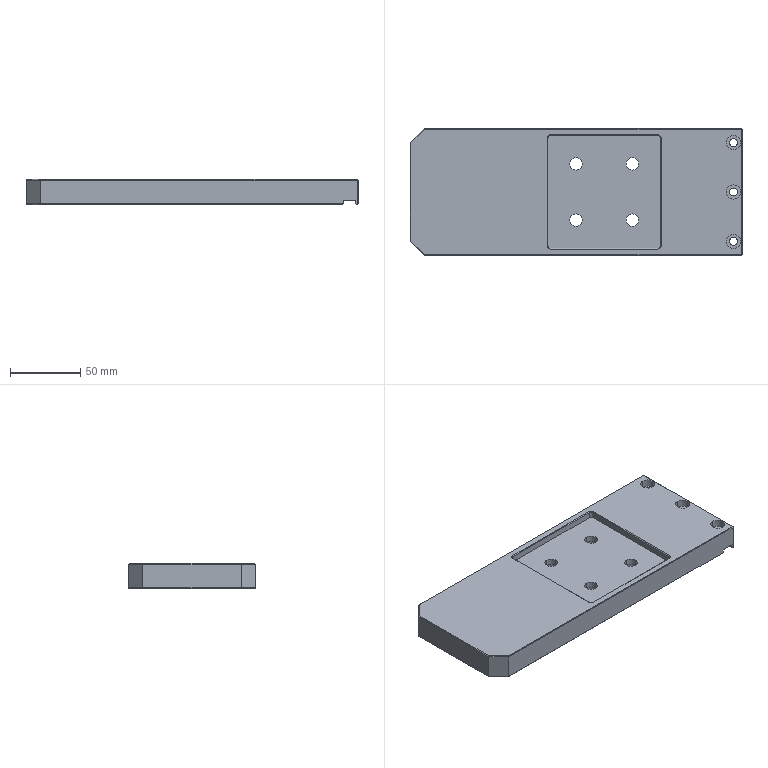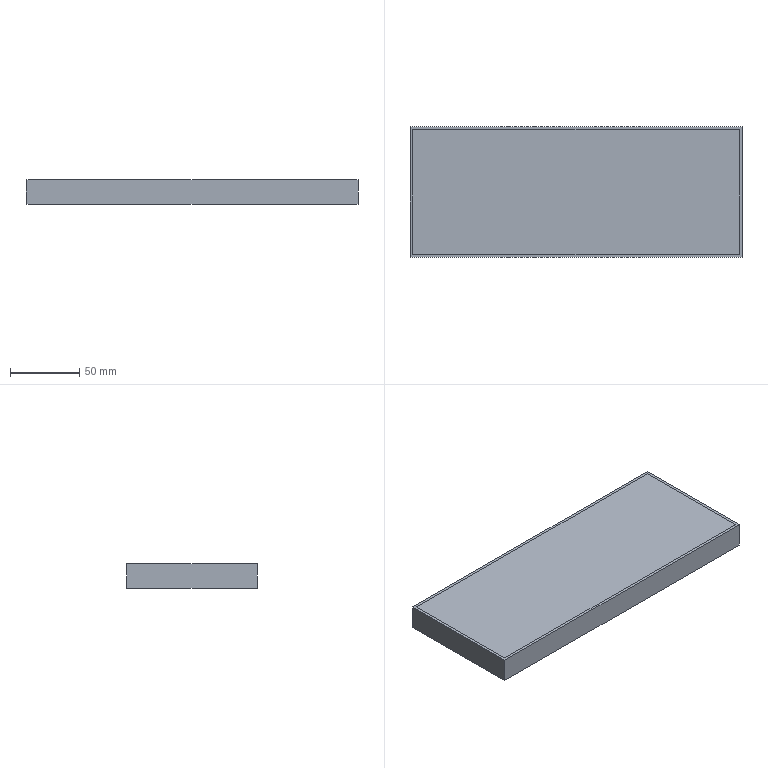CAM job | NX | 3-axis milling, drilling | part box 235.5 x 90 x 18 mm | stock box 239.5 x 94 x 18 mm
Tools:
number,name,description,diameter,corner_radius,flute_length,length,flutes
1,D6A45,Milling Tool-5 Parameters,6.0,0.0,50.0,75.0,2
9,5.5ZT,Drilling Tool,5.5,0.0,35.0,50.0,2
16,9.0ZT,Drilling Tool,9.0,0.0,35.0,50.0,2
15,D10,Milling Tool-5 Parameters,10.0,0.0,50.0,75.0,2
14,D10JING,Milling Tool-5 Parameters,10.0,0.0,50.0,75.0,2
6,D6,Milling Tool-5 Parameters,6.0,0.0,50.0,75.0,2
11,D4,Milling Tool-5 Parameters,4.0,0.0,50.0,75.0,2
Operations:
program,operation,operation_type,tool,method,geometry_group,spindle_rpm,surface_speed,feed_per_tooth,feed_cut,feed_plunge,cut_length_mm,path_length_mm,cut_time_min,machine_time_min
1,DRILLING,Operation,D6A45,METHOD,A,5000.0,94.0,0.025,250.0,0.0,35.0,411.956,0.14,0.1777
1,DRILLING_1,Operation,5.5ZT,METHOD,A,2000.0,34.0,0.05,200.0,0.0,72.457,281.171,0.3623,0.3832
1,DRILLING_1_COPY,Operation,9.0ZT,METHOD,A,2000.0,34.0,0.05,200.0,0.0,100.816,390.968,0.5041,0.5331
1,ZLEVEL_PROFILE,ZLevelMilling,D10,METHOD,A,9500.0,298.0,0.1842,3500.0,1000.0,12792.536,12866.936,3.689,3.696
1,FLOOR_WALL,VolumeBased25DMillingOperation,D10,METHOD,A,9500.0,298.0,0.1842,3500.0,1000.0,4705.431,4906.327,1.53,1.55
1,HOLE_MILLING,CylinderMilling,D6,METHOD,A,9500.0,179.0,0.0789,1500.0,100.0,427.679,692.379,0.2851,0.3116
1,ZLEVEL_PROFILE_COPY_1,ZLevelMilling,D4,METHOD,A,9500.0,119.0,0.1053,2000.0,1000.0,384.836,1028.795,0.2191,0.2835
1,PLANAR_MILL,PlanarMilling,D6A45,METHOD,A,9500.0,179.0,0.0789,1500.0,100.0,109.46,511.965,0.073,0.1132
1,PLANAR_MILL_COPY,PlanarMilling,D6A45,METHOD,A,9500.0,179.0,0.0789,1500.0,100.0,91.29,348.051,0.0609,0.0865
1,PLANAR_MILL_COPY_COPY,PlanarMilling,D6A45,METHOD,A,9500.0,179.0,0.0789,1500.0,100.0,963.524,1100.21,0.6423,0.656
1,FLOOR_WALL_COPY,VolumeBased25DMillingOperation,D10JING,METHOD,A,9500.0,298.0,0.0789,1500.0,1000.0,1471.322,1570.148,1.002,1.011
1,ZLEVEL_PROFILE_COPY,ZLevelMilling,D10JING,METHOD,A,9500.0,298.0,0.0789,1500.0,1000.0,3724.908,3783.208,2.602,2.608
2,HOLE_MILLING_COPY,CylinderMilling,D6,METHOD,B,9500.0,179.0,0.0789,1500.0,100.0,2828.592,3257.392,1.886,1.929
2,FLOOR_WALL_COPY_1,VolumeBased25DMillingOperation,D6,METHOD,B,9500.0,298.0,0.1842,3500.0,1000.0,2432.315,2566.96,0.7168,0.7303
2,FLOOR_WALL_COPY_COPY,VolumeBased25DMillingOperation,D6,METHOD,B,9500.0,298.0,0.0789,1500.0,1000.0,402.508,471.264,0.2702,0.2771
2,PLANAR_MILL_COPY_1,PlanarMilling,D6A45,METHOD,B,9500.0,179.0,0.0789,1500.0,100.0,183.905,545.938,0.1226,0.1588
2,PLANAR_MILL_COPY_1_COPY,PlanarMilling,D6A45,METHOD,B,9500.0,179.0,0.0789,1500.0,100.0,625.236,685.236,0.4168,0.4228
2,PLANAR_MILL_COPY_1_COPY_COPY,PlanarMilling,D6A45,METHOD,B,9500.0,179.0,0.0526,1000.0,100.0,191.361,251.361,0.1914,0.1974